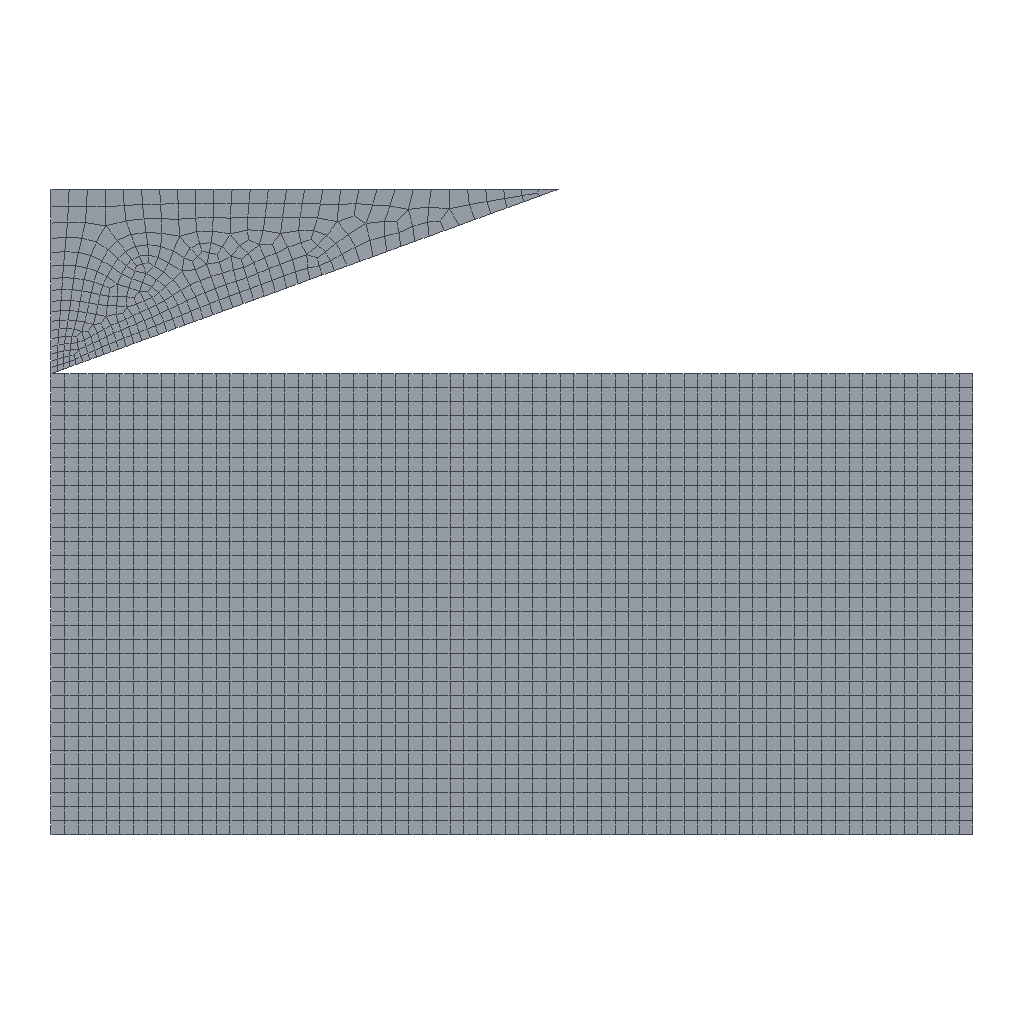Simulation study | abaqus
Set-up summary:
category,name,step,type,value,unit,region
solver,abaqus
solver,version,,,Abaqus/Standard 2020
units,not stated in the deck,,not stated
analysis,deck,,static,static
load_step,Step-1,Step-1,static
load_step,Step-2,Step-2,transient
load_step,requested,,,2
mesh,nodes,,,2688
mesh,elements,,,2540
element_type,CPE4,,plane,2211
element_type,CPS4R,,plane,329
load,load commands in deck,,count,1
bc,support commands in deck,,count,5
material,TOOL,,in results
material,WORK,,in results
check,setup vs results,,match,"per instance, exact: element labels, types and connectivity; labels of the nodes the elements use; coordinates of those nodes at SINGLE_PRECISION in 2 of 2 instance(s)"
Abaqus input file, long lists of numbers shortened:
*Heading
** Job name: Job-2 Model name: Model-1
** Generated by: Abaqus/CAE 2020
*Preprint, echo=NO, model=NO, history=NO, contact=NO
**
** PARTS
**
*Part, name=tou
*Node
      1,           0.,         -20.
      2,           0.,           0.
** (374 more lines like these left out)
*Element, type=CPS4R
  1, 321, 338, 339, 359
  2,   4,   1,  65,  93
** (327 more lines like these left out)
*Nset, nset=Set-1, generate
   1,  376,    1
*Elset, elset=Set-1, generate
   1,  329,    1
** Section: Section-2
*Solid Section, elset=Set-1, material=tool
,
*End Part
**
*Part, name=work
*Node
      1,         100.,           0.
      2,   98.507,           0.
** (2310 more lines like these left out)
*Element, type=CPE4
   1,    1,    2,   70,   69
   2,    2,    3,   71,   70
** (2209 more lines like these left out)
*Nset, nset=Set-1, generate
    1,  2312,     1
*Elset, elset=Set-1, generate
    1,  2211,     1
** Section: Section-1
*Solid Section, elset=Set-1, material=work
,
*End Part
**
**
** ASSEMBLY
**
*Assembly, name=Assembly
**
*Instance, name=tou-1, part=tou
          0.,          20.,           0.
*End Instance
**
*Instance, name=work-1, part=work
*End Instance
**
*Node
      1,           0.,          20.,           0.
*Nset, nset=Set-3, instance=work-1, generate
 2245,  2312,     1
*Elset, elset=Set-3, instance=work-1, generate
 2145,  2211,     1
*Nset, nset=Set-4
 1,
*Nset, nset=Set-5, instance=work-1, generate
   68,  2312,    68
*Elset, elset=Set-5, instance=work-1, generate
   67,  2211,    67
*Nset, nset=b_Set-1, instance=tou-1, generate
   1,  376,    1
*Elset, elset=b_Set-1, instance=tou-1, generate
   1,  329,    1
*Nset, nset=_PickedSet8, internal
 1,
*Elset, elset=_m_Surf-1_S1, internal, instance=tou-1
   2,   5,   6,   8,  11,  12,  13,  14,  15,  17,  18,  20,  55,  82,  83, 270
 298, 300, 302, 326
*Elset, elset=_m_Surf-1_S3, internal, instance=tou-1
  4, 23, 56, 76, 77, 80
*Elset, elset=_m_Surf-1_S2, internal, instance=tou-1
   2,   3,   9,  17,  22,  54,  79,  94, 112, 119, 120, 122, 279, 289, 295, 301
 312, 317, 321, 322, 323, 324, 325
*Elset, elset=_m_Surf-1_S4, internal, instance=tou-1
  19,  21,  24,  25,  26,  27,  28,  29,  30,  31,  32,  33,  34,  35,  36,  37
  38,  39,  40,  41,  42,  43,  44,  45,  46,  47,  48,  49,  50,  51,  55,  78
** (1 more lines like these left out)
*Surface, type=ELEMENT, name=m_Surf-1
_m_Surf-1_S1, S1
_m_Surf-1_S3, S3
_m_Surf-1_S2, S2
_m_Surf-1_S4, S4
*Elset, elset=_s_Surf-1_S1, internal, instance=work-1, generate
  1,  67,   1
*Elset, elset=_s_Surf-1_S2, internal, instance=work-1, generate
   67,  2211,    67
*Surface, type=ELEMENT, name=s_Surf-1
_s_Surf-1_S1, S1
_s_Surf-1_S2, S2
** Constraint: Constraint-1
*Rigid Body, ref node=_PickedSet8, elset=b_Set-1, position=CENTER OF MASS
*End Assembly
*Amplitude, name=Amp-1
             0.,              0.,              1.,              1.
**
** MATERIALS
**
*Material, name=tool
*Density
 7.8e-09,
*Elastic
210000., 0.3
*Material, name=work
*Creep
 0.01, 0.8, 0.5
*Elastic
1000., 0.4
*Plastic
50.,0.
**
** INTERACTION PROPERTIES
**
*Surface Interaction, name=IntProp-1
1.,
*Friction, slip tolerance=0.005
 0.2,
*Surface Behavior, pressure-overclosure=HARD
**
** INTERACTIONS
**
** Interaction: Int-1
*Contact Pair, interaction=IntProp-1, type=SURFACE TO SURFACE
s_Surf-1, m_Surf-1
** ----------------------------------------------------------------
**
** STEP: Step-1
**
*Step, name=Step-1, nlgeom=YES
*Static, stabilize=0.0002, allsdtol=0.05, continue=NO
0.01, 1., 1e-05, 1.
**
** BOUNDARY CONDITIONS
**
** Name: BC-1 Type: 对称/反对称/完全固定
*Boundary
Set-3, ENCASTRE
** Name: BC-2 Type: 位移/转角
*Boundary, amplitude=Amp-1
Set-4, 1, 1
Set-4, 2, 2, -5.
Set-4, 6, 6
** Name: BC-3 Type: 对称/反对称/完全固定
*Boundary
Set-5, XSYMM
**
** OUTPUT REQUESTS
**
*Restart, write, frequency=0
**
** FIELD OUTPUT: F-Output-1
**
*Output, field
*Node Output
CF, RF, U, V
*Element Output, directions=YES
E, LE, MISES, MISESMAX, PE, PEEQ, PEEQT, S, VE, VEEQ, VS
*Contact Output
CDISP, CSTRESS
**
** HISTORY OUTPUT: H-Output-1
**
*Output, history, variable=PRESELECT
*End Step
** ----------------------------------------------------------------
**
** STEP: Step-2
**
*Step, name=Step-2, nlgeom=YES, inc=10000
*Visco, cetol=1.
0.0001, 50., 5e-06, 50.
**
** OUTPUT REQUESTS
**
*Restart, write, frequency=0
**
** FIELD OUTPUT: F-Output-1
**
*Output, field
*Node Output
CF, RF, U, V
*Element Output, directions=YES
CE, CEEQ, CEMAG, CEP, E, LE, MISES, MISESMAX, PE, PEEQ, PEEQT, S, VE, VEEQ, VS
*Contact Output
CDISP, CSTRESS
**
** HISTORY OUTPUT: H-Output-1
**
*Output, history, variable=PRESELECT
*End Step
Results summary:
result,step,,completed,increments=17 time=1.0/1.0
result,step,,partial,increments=340 time=1.02/50.0
result,analysis,,,transient
result,last_loadstep,,,2
result,primary field,,,U
result,reaction total,,FX,-2e-06,model units
result,reaction total,,FY,-1e-06,model units
result,reaction total,,FZ,0.0,model units